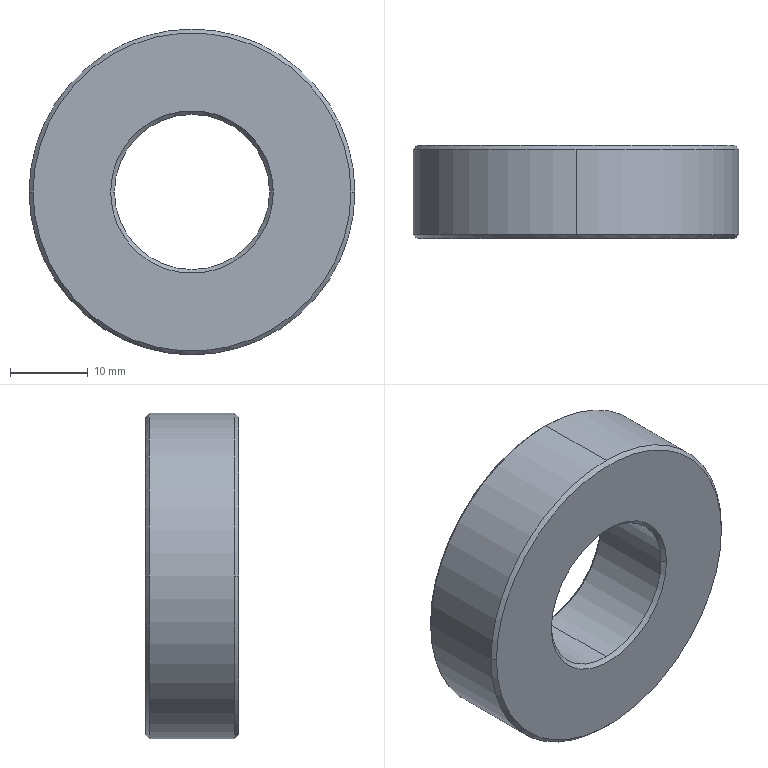Part | SolidWorks | features BaseBody 1 | 1 solid | 14 faces | box 42 x 12 x 42 mm | volume 12807 mm3 | cone 8 | cylinder 4 | plane 2 | commonest cylinder face diameters 20 x2 42 x2
STEP:
#1=CARTESIAN_POINT('',(10.,5.5,0.));
#2=VERTEX_POINT('',#1);
#3=CARTESIAN_POINT('',(0.,5.5,-10.));
#4=VERTEX_POINT('',#3);
#5=CARTESIAN_POINT('',(0.,5.5,0.));
#6=DIRECTION('',(0.,1.,0.));
#7=DIRECTION('',(0.,0.,-1.));
#8=AXIS2_PLACEMENT_3D('',#5,#6,#7);
#9=CIRCLE('',#8,10.);
#10=EDGE_CURVE('',#2,#4,#9,.T.);
#11=ORIENTED_EDGE('',*,*,#10,.F.);
#12=CARTESIAN_POINT('',(10.5,6.,0.));
#13=VERTEX_POINT('',#12);
#14=CARTESIAN_POINT('',(10.5,6.,0.));
#15=DIRECTION('',(0.7071,0.7071,0.));
#16=VECTOR('',#15,1000.);
#17=LINE('',#14,#16);
#18=EDGE_CURVE('',#2,#13,#17,.T.);
#19=ORIENTED_EDGE('',*,*,#18,.T.);
#20=CARTESIAN_POINT('',(-10.5,6.,0.));
#21=VERTEX_POINT('',#20);
#22=CARTESIAN_POINT('',(0.,6.,0.));
#23=DIRECTION('',(0.,-1.,0.));
#24=DIRECTION('',(-1.,0.,0.));
#25=AXIS2_PLACEMENT_3D('',#22,#23,#24);
#26=CIRCLE('',#25,10.5);
#27=EDGE_CURVE('',#21,#13,#26,.T.);
#28=ORIENTED_EDGE('',*,*,#27,.F.);
#29=CARTESIAN_POINT('',(-10.,5.5,0.));
#30=VERTEX_POINT('',#29);
#31=CARTESIAN_POINT('',(-10.5,6.,0.));
#32=DIRECTION('',(-0.7071,0.7071,0.));
#33=VECTOR('',#32,1000.);
#34=LINE('',#31,#33);
#35=EDGE_CURVE('',#30,#21,#34,.T.);
#36=ORIENTED_EDGE('',*,*,#35,.F.);
#37=CARTESIAN_POINT('',(0.,5.5,0.));
#38=DIRECTION('',(0.,1.,0.));
#39=DIRECTION('',(0.,0.,-1.));
#40=AXIS2_PLACEMENT_3D('',#37,#38,#39);
#41=CIRCLE('',#40,10.);
#42=EDGE_CURVE('',#4,#30,#41,.T.);
#43=ORIENTED_EDGE('',*,*,#42,.F.);
#44=EDGE_LOOP('',(#11,#19,#28,#36,#43));
#45=FACE_OUTER_BOUND('',#44,.T.);
#46=CARTESIAN_POINT('',(0.,6.,0.));
#47=DIRECTION('',(0.,1.,0.));
#48=DIRECTION('',(-1.,0.,0.));
#49=AXIS2_PLACEMENT_3D('',#46,#47,#48);
#50=CONICAL_SURFACE('',#49,10.5,0.7854);
#51=ADVANCED_FACE('',(#45),#50,.F.);
#52=CARTESIAN_POINT('',(-20.5,6.,0.));
#53=VERTEX_POINT('',#52);
#54=CARTESIAN_POINT('',(20.5,6.,0.));
#55=VERTEX_POINT('',#54);
#56=CARTESIAN_POINT('',(0.,6.,0.));
#57=DIRECTION('',(0.,1.,0.));
#58=DIRECTION('',(1.,0.,0.));
#59=AXIS2_PLACEMENT_3D('',#56,#57,#58);
#60=CIRCLE('',#59,20.5);
#61=EDGE_CURVE('',#53,#55,#60,.T.);
#62=ORIENTED_EDGE('',*,*,#61,.F.);
#63=CARTESIAN_POINT('',(-21.,5.5,0.));
#64=VERTEX_POINT('',#63);
#65=CARTESIAN_POINT('',(-21.,5.5,0.));
#66=DIRECTION('',(-0.7071,-0.7071,0.));
#67=VECTOR('',#66,1000.);
#68=LINE('',#65,#67);
#69=EDGE_CURVE('',#53,#64,#68,.T.);
#70=ORIENTED_EDGE('',*,*,#69,.T.);
#71=CARTESIAN_POINT('',(0.,5.5,21.));
#72=VERTEX_POINT('',#71);
#73=CARTESIAN_POINT('',(0.,5.5,0.));
#74=DIRECTION('',(0.,1.,0.));
#75=DIRECTION('',(0.,0.,-1.));
#76=AXIS2_PLACEMENT_3D('',#73,#74,#75);
#77=CIRCLE('',#76,21.);
#78=EDGE_CURVE('',#64,#72,#77,.T.);
#79=ORIENTED_EDGE('',*,*,#78,.T.);
#80=CARTESIAN_POINT('',(21.,5.5,0.));
#81=VERTEX_POINT('',#80);
#82=CARTESIAN_POINT('',(0.,5.5,0.));
#83=DIRECTION('',(0.,1.,0.));
#84=DIRECTION('',(0.,0.,-1.));
#85=AXIS2_PLACEMENT_3D('',#82,#83,#84);
#86=CIRCLE('',#85,21.);
#87=EDGE_CURVE('',#72,#81,#86,.T.);
#88=ORIENTED_EDGE('',*,*,#87,.T.);
#89=CARTESIAN_POINT('',(21.,5.5,0.));
#90=DIRECTION('',(0.7071,-0.7071,0.));
#91=VECTOR('',#90,1000.);
#92=LINE('',#89,#91);
#93=EDGE_CURVE('',#55,#81,#92,.T.);
#94=ORIENTED_EDGE('',*,*,#93,.F.);
#95=EDGE_LOOP('',(#62,#70,#79,#88,#94));
#96=FACE_OUTER_BOUND('',#95,.T.);
#97=CARTESIAN_POINT('',(0.,5.5,0.));
#98=DIRECTION('',(0.,-1.,0.));
#99=DIRECTION('',(1.,0.,0.));
#100=AXIS2_PLACEMENT_3D('',#97,#98,#99);
#101=CONICAL_SURFACE('',#100,21.,0.7854);
#102=ADVANCED_FACE('',(#96),#101,.T.);
#103=CARTESIAN_POINT('',(0.,-5.5,-10.));
#104=VERTEX_POINT('',#103);
#105=CARTESIAN_POINT('',(-10.,-5.5,0.));
#106=VERTEX_POINT('',#105);
#107=CARTESIAN_POINT('',(0.,-5.5,0.));
#108=DIRECTION('',(0.,1.,0.));
#109=DIRECTION('',(0.,0.,1.));
#110=AXIS2_PLACEMENT_3D('',#107,#108,#109);
#111=CIRCLE('',#110,10.);
#112=EDGE_CURVE('',#104,#106,#111,.T.);
#113=ORIENTED_EDGE('',*,*,#112,.F.);
#114=CARTESIAN_POINT('',(0.,-6.,-10.));
#115=DIRECTION('',(0.,1.,0.));
#116=VECTOR('',#115,1000.);
#117=LINE('',#114,#116);
#118=EDGE_CURVE('',#104,#4,#117,.T.);
#119=ORIENTED_EDGE('',*,*,#118,.T.);
#120=ORIENTED_EDGE('',*,*,#42,.T.);
#121=CARTESIAN_POINT('',(0.,5.5,10.));
#122=VERTEX_POINT('',#121);
#123=CARTESIAN_POINT('',(0.,5.5,0.));
#124=DIRECTION('',(0.,1.,0.));
#125=DIRECTION('',(0.,0.,-1.));
#126=AXIS2_PLACEMENT_3D('',#123,#124,#125);
#127=CIRCLE('',#126,10.);
#128=EDGE_CURVE('',#30,#122,#127,.T.);
#129=ORIENTED_EDGE('',*,*,#128,.T.);
#130=CARTESIAN_POINT('',(0.,-5.5,10.));
#131=VERTEX_POINT('',#130);
#132=CARTESIAN_POINT('',(0.,-6.,10.));
#133=DIRECTION('',(0.,1.,0.));
#134=VECTOR('',#133,1000.);
#135=LINE('',#132,#134);
#136=EDGE_CURVE('',#131,#122,#135,.T.);
#137=ORIENTED_EDGE('',*,*,#136,.F.);
#138=CARTESIAN_POINT('',(0.,-5.5,0.));
#139=DIRECTION('',(0.,1.,0.));
#140=DIRECTION('',(0.,0.,1.));
#141=AXIS2_PLACEMENT_3D('',#138,#139,#140);
#142=CIRCLE('',#141,10.);
#143=EDGE_CURVE('',#106,#131,#142,.T.);
#144=ORIENTED_EDGE('',*,*,#143,.F.);
#145=EDGE_LOOP('',(#113,#119,#120,#129,#137,#144));
#146=FACE_OUTER_BOUND('',#145,.T.);
#147=CARTESIAN_POINT('',(0.,-6.,0.));
#148=DIRECTION('',(0.,1.,0.));
#149=DIRECTION('',(0.,0.,1.));
#150=AXIS2_PLACEMENT_3D('',#147,#148,#149);
#151=CYLINDRICAL_SURFACE('',#150,10.);
#152=ADVANCED_FACE('',(#146),#151,.F.);
#153=CARTESIAN_POINT('',(21.,-5.5,0.));
#154=VERTEX_POINT('',#153);
#155=CARTESIAN_POINT('',(0.,-5.5,-21.));
#156=VERTEX_POINT('',#155);
#157=CARTESIAN_POINT('',(0.,-5.5,0.));
#158=DIRECTION('',(0.,1.,0.));
#159=DIRECTION('',(0.,0.,1.));
#160=AXIS2_PLACEMENT_3D('',#157,#158,#159);
#161=CIRCLE('',#160,21.);
#162=EDGE_CURVE('',#154,#156,#161,.T.);
#163=ORIENTED_EDGE('',*,*,#162,.T.);
#164=CARTESIAN_POINT('',(0.,5.5,-21.));
#165=VERTEX_POINT('',#164);
#166=CARTESIAN_POINT('',(0.,-6.,-21.));
#167=DIRECTION('',(0.,1.,0.));
#168=VECTOR('',#167,1000.);
#169=LINE('',#166,#168);
#170=EDGE_CURVE('',#156,#165,#169,.T.);
#171=ORIENTED_EDGE('',*,*,#170,.T.);
#172=CARTESIAN_POINT('',(0.,5.5,0.));
#173=DIRECTION('',(0.,1.,0.));
#174=DIRECTION('',(0.,0.,-1.));
#175=AXIS2_PLACEMENT_3D('',#172,#173,#174);
#176=CIRCLE('',#175,21.);
#177=EDGE_CURVE('',#81,#165,#176,.T.);
#178=ORIENTED_EDGE('',*,*,#177,.F.);
#179=ORIENTED_EDGE('',*,*,#87,.F.);
#180=CARTESIAN_POINT('',(0.,-5.5,21.));
#181=VERTEX_POINT('',#180);
#182=CARTESIAN_POINT('',(0.,-6.,21.));
#183=DIRECTION('',(0.,1.,0.));
#184=VECTOR('',#183,1000.);
#185=LINE('',#182,#184);
#186=EDGE_CURVE('',#181,#72,#185,.T.);
#187=ORIENTED_EDGE('',*,*,#186,.F.);
#188=CARTESIAN_POINT('',(0.,-5.5,0.));
#189=DIRECTION('',(0.,1.,0.));
#190=DIRECTION('',(0.,0.,1.));
#191=AXIS2_PLACEMENT_3D('',#188,#189,#190);
#192=CIRCLE('',#191,21.);
#193=EDGE_CURVE('',#181,#154,#192,.T.);
#194=ORIENTED_EDGE('',*,*,#193,.T.);
#195=EDGE_LOOP('',(#163,#171,#178,#179,#187,#194));
#196=FACE_OUTER_BOUND('',#195,.T.);
#197=CARTESIAN_POINT('',(0.,-6.,0.));
#198=DIRECTION('',(0.,1.,0.));
#199=DIRECTION('',(0.,0.,1.));
#200=AXIS2_PLACEMENT_3D('',#197,#198,#199);
#201=CYLINDRICAL_SURFACE('',#200,21.);
#202=ADVANCED_FACE('',(#196),#201,.T.);
#203=CARTESIAN_POINT('',(10.,-5.5,0.));
#204=VERTEX_POINT('',#203);
#205=CARTESIAN_POINT('',(0.,-5.5,0.));
#206=DIRECTION('',(0.,1.,0.));
#207=DIRECTION('',(0.,0.,1.));
#208=AXIS2_PLACEMENT_3D('',#205,#206,#207);
#209=CIRCLE('',#208,10.);
#210=EDGE_CURVE('',#204,#104,#209,.T.);
#211=ORIENTED_EDGE('',*,*,#210,.T.);
#212=ORIENTED_EDGE('',*,*,#112,.T.);
#213=CARTESIAN_POINT('',(-10.5,-6.,0.));
#214=VERTEX_POINT('',#213);
#215=CARTESIAN_POINT('',(-10.5,-6.,0.));
#216=DIRECTION('',(-0.7071,-0.7071,0.));
#217=VECTOR('',#216,1000.);
#218=LINE('',#215,#217);
#219=EDGE_CURVE('',#106,#214,#218,.T.);
#220=ORIENTED_EDGE('',*,*,#219,.T.);
#221=CARTESIAN_POINT('',(10.5,-6.,0.));
#222=VERTEX_POINT('',#221);
#223=CARTESIAN_POINT('',(0.,-6.,0.));
#224=DIRECTION('',(0.,1.,0.));
#225=DIRECTION('',(1.,0.,0.));
#226=AXIS2_PLACEMENT_3D('',#223,#224,#225);
#227=CIRCLE('',#226,10.5);
#228=EDGE_CURVE('',#222,#214,#227,.T.);
#229=ORIENTED_EDGE('',*,*,#228,.F.);
#230=CARTESIAN_POINT('',(10.5,-6.,0.));
#231=DIRECTION('',(0.7071,-0.7071,0.));
#232=VECTOR('',#231,1000.);
#233=LINE('',#230,#232);
#234=EDGE_CURVE('',#204,#222,#233,.T.);
#235=ORIENTED_EDGE('',*,*,#234,.F.);
#236=EDGE_LOOP('',(#211,#212,#220,#229,#235));
#237=FACE_OUTER_BOUND('',#236,.T.);
#238=CARTESIAN_POINT('',(0.,-6.,0.));
#239=DIRECTION('',(0.,-1.,0.));
#240=DIRECTION('',(1.,0.,0.));
#241=AXIS2_PLACEMENT_3D('',#238,#239,#240);
#242=CONICAL_SURFACE('',#241,10.5,0.7854);
#243=ADVANCED_FACE('',(#237),#242,.F.);
#244=CARTESIAN_POINT('',(-20.5,-6.,0.));
#245=VERTEX_POINT('',#244);
#246=CARTESIAN_POINT('',(20.5,-6.,0.));
#247=VERTEX_POINT('',#246);
#248=CARTESIAN_POINT('',(0.,-6.,0.));
#249=DIRECTION('',(0.,1.,0.));
#250=DIRECTION('',(-1.,0.,0.));
#251=AXIS2_PLACEMENT_3D('',#248,#249,#250);
#252=CIRCLE('',#251,20.5);
#253=EDGE_CURVE('',#245,#247,#252,.T.);
#254=ORIENTED_EDGE('',*,*,#253,.T.);
#255=CARTESIAN_POINT('',(21.,-5.5,0.));
#256=DIRECTION('',(0.7071,0.7071,0.));
#257=VECTOR('',#256,1000.);
#258=LINE('',#255,#257);
#259=EDGE_CURVE('',#247,#154,#258,.T.);
#260=ORIENTED_EDGE('',*,*,#259,.T.);
#261=ORIENTED_EDGE('',*,*,#193,.F.);
#262=CARTESIAN_POINT('',(-21.,-5.5,0.));
#263=VERTEX_POINT('',#262);
#264=CARTESIAN_POINT('',(0.,-5.5,0.));
#265=DIRECTION('',(0.,1.,0.));
#266=DIRECTION('',(0.,0.,1.));
#267=AXIS2_PLACEMENT_3D('',#264,#265,#266);
#268=CIRCLE('',#267,21.);
#269=EDGE_CURVE('',#263,#181,#268,.T.);
#270=ORIENTED_EDGE('',*,*,#269,.F.);
#271=CARTESIAN_POINT('',(-21.,-5.5,0.));
#272=DIRECTION('',(-0.7071,0.7071,0.));
#273=VECTOR('',#272,1000.);
#274=LINE('',#271,#273);
#275=EDGE_CURVE('',#245,#263,#274,.T.);
#276=ORIENTED_EDGE('',*,*,#275,.F.);
#277=EDGE_LOOP('',(#254,#260,#261,#270,#276));
#278=FACE_OUTER_BOUND('',#277,.T.);
#279=CARTESIAN_POINT('',(0.,-5.5,0.));
#280=DIRECTION('',(0.,1.,0.));
#281=DIRECTION('',(-1.,0.,0.));
#282=AXIS2_PLACEMENT_3D('',#279,#280,#281);
#283=CONICAL_SURFACE('',#282,21.,0.7854);
#284=ADVANCED_FACE('',(#278),#283,.T.);
#285=ORIENTED_EDGE('',*,*,#27,.T.);
#286=CARTESIAN_POINT('',(0.,6.,0.));
#287=DIRECTION('',(0.,-1.,0.));
#288=DIRECTION('',(-1.,0.,0.));
#289=AXIS2_PLACEMENT_3D('',#286,#287,#288);
#290=CIRCLE('',#289,10.5);
#291=EDGE_CURVE('',#13,#21,#290,.T.);
#292=ORIENTED_EDGE('',*,*,#291,.T.);
#293=EDGE_LOOP('',(#285,#292));
#294=FACE_BOUND('',#293,.T.);
#295=CARTESIAN_POINT('',(0.,6.,0.));
#296=DIRECTION('',(0.,1.,0.));
#297=DIRECTION('',(1.,0.,0.));
#298=AXIS2_PLACEMENT_3D('',#295,#296,#297);
#299=CIRCLE('',#298,20.5);
#300=EDGE_CURVE('',#55,#53,#299,.T.);
#301=ORIENTED_EDGE('',*,*,#300,.T.);
#302=ORIENTED_EDGE('',*,*,#61,.T.);
#303=EDGE_LOOP('',(#301,#302));
#304=FACE_OUTER_BOUND('',#303,.T.);
#305=CARTESIAN_POINT('',(0.,6.,0.));
#306=DIRECTION('',(0.,1.,0.));
#307=DIRECTION('',(0.,0.,1.));
#308=AXIS2_PLACEMENT_3D('',#305,#306,#307);
#309=PLANE('',#308);
#310=ADVANCED_FACE('',(#294,#304),#309,.T.);
#311=ORIENTED_EDGE('',*,*,#18,.F.);
#312=CARTESIAN_POINT('',(0.,5.5,0.));
#313=DIRECTION('',(0.,1.,0.));
#314=DIRECTION('',(0.,0.,-1.));
#315=AXIS2_PLACEMENT_3D('',#312,#313,#314);
#316=CIRCLE('',#315,10.);
#317=EDGE_CURVE('',#122,#2,#316,.T.);
#318=ORIENTED_EDGE('',*,*,#317,.F.);
#319=ORIENTED_EDGE('',*,*,#128,.F.);
#320=ORIENTED_EDGE('',*,*,#35,.T.);
#321=ORIENTED_EDGE('',*,*,#291,.F.);
#322=EDGE_LOOP('',(#311,#318,#319,#320,#321));
#323=FACE_OUTER_BOUND('',#322,.T.);
#324=CARTESIAN_POINT('',(0.,6.,0.));
#325=DIRECTION('',(0.,1.,0.));
#326=DIRECTION('',(-1.,0.,0.));
#327=AXIS2_PLACEMENT_3D('',#324,#325,#326);
#328=CONICAL_SURFACE('',#327,10.5,0.7854);
#329=ADVANCED_FACE('',(#323),#328,.F.);
#330=ORIENTED_EDGE('',*,*,#69,.F.);
#331=ORIENTED_EDGE('',*,*,#300,.F.);
#332=ORIENTED_EDGE('',*,*,#93,.T.);
#333=ORIENTED_EDGE('',*,*,#177,.T.);
#334=CARTESIAN_POINT('',(0.,5.5,0.));
#335=DIRECTION('',(0.,1.,0.));
#336=DIRECTION('',(0.,0.,-1.));
#337=AXIS2_PLACEMENT_3D('',#334,#335,#336);
#338=CIRCLE('',#337,21.);
#339=EDGE_CURVE('',#165,#64,#338,.T.);
#340=ORIENTED_EDGE('',*,*,#339,.T.);
#341=EDGE_LOOP('',(#330,#331,#332,#333,#340));
#342=FACE_OUTER_BOUND('',#341,.T.);
#343=CARTESIAN_POINT('',(0.,5.5,0.));
#344=DIRECTION('',(0.,-1.,0.));
#345=DIRECTION('',(1.,0.,0.));
#346=AXIS2_PLACEMENT_3D('',#343,#344,#345);
#347=CONICAL_SURFACE('',#346,21.,0.7854);
#348=ADVANCED_FACE('',(#342),#347,.T.);
#349=ORIENTED_EDGE('',*,*,#118,.F.);
#350=ORIENTED_EDGE('',*,*,#210,.F.);
#351=CARTESIAN_POINT('',(0.,-5.5,0.));
#352=DIRECTION('',(0.,1.,0.));
#353=DIRECTION('',(0.,0.,1.));
#354=AXIS2_PLACEMENT_3D('',#351,#352,#353);
#355=CIRCLE('',#354,10.);
#356=EDGE_CURVE('',#131,#204,#355,.T.);
#357=ORIENTED_EDGE('',*,*,#356,.F.);
#358=ORIENTED_EDGE('',*,*,#136,.T.);
#359=ORIENTED_EDGE('',*,*,#317,.T.);
#360=ORIENTED_EDGE('',*,*,#10,.T.);
#361=EDGE_LOOP('',(#349,#350,#357,#358,#359,#360));
#362=FACE_OUTER_BOUND('',#361,.T.);
#363=CARTESIAN_POINT('',(0.,-6.,0.));
#364=DIRECTION('',(0.,1.,0.));
#365=DIRECTION('',(0.,0.,1.));
#366=AXIS2_PLACEMENT_3D('',#363,#364,#365);
#367=CYLINDRICAL_SURFACE('',#366,10.);
#368=ADVANCED_FACE('',(#362),#367,.F.);
#369=ORIENTED_EDGE('',*,*,#170,.F.);
#370=CARTESIAN_POINT('',(0.,-5.5,0.));
#371=DIRECTION('',(0.,1.,0.));
#372=DIRECTION('',(0.,0.,1.));
#373=AXIS2_PLACEMENT_3D('',#370,#371,#372);
#374=CIRCLE('',#373,21.);
#375=EDGE_CURVE('',#156,#263,#374,.T.);
#376=ORIENTED_EDGE('',*,*,#375,.T.);
#377=ORIENTED_EDGE('',*,*,#269,.T.);
#378=ORIENTED_EDGE('',*,*,#186,.T.);
#379=ORIENTED_EDGE('',*,*,#78,.F.);
#380=ORIENTED_EDGE('',*,*,#339,.F.);
#381=EDGE_LOOP('',(#369,#376,#377,#378,#379,#380));
#382=FACE_OUTER_BOUND('',#381,.T.);
#383=CARTESIAN_POINT('',(0.,-6.,0.));
#384=DIRECTION('',(0.,1.,0.));
#385=DIRECTION('',(0.,0.,1.));
#386=AXIS2_PLACEMENT_3D('',#383,#384,#385);
#387=CYLINDRICAL_SURFACE('',#386,21.);
#388=ADVANCED_FACE('',(#382),#387,.T.);
#389=ORIENTED_EDGE('',*,*,#219,.F.);
#390=ORIENTED_EDGE('',*,*,#143,.T.);
#391=ORIENTED_EDGE('',*,*,#356,.T.);
#392=ORIENTED_EDGE('',*,*,#234,.T.);
#393=CARTESIAN_POINT('',(0.,-6.,0.));
#394=DIRECTION('',(0.,1.,0.));
#395=DIRECTION('',(1.,0.,0.));
#396=AXIS2_PLACEMENT_3D('',#393,#394,#395);
#397=CIRCLE('',#396,10.5);
#398=EDGE_CURVE('',#214,#222,#397,.T.);
#399=ORIENTED_EDGE('',*,*,#398,.F.);
#400=EDGE_LOOP('',(#389,#390,#391,#392,#399));
#401=FACE_OUTER_BOUND('',#400,.T.);
#402=CARTESIAN_POINT('',(0.,-6.,0.));
#403=DIRECTION('',(0.,-1.,0.));
#404=DIRECTION('',(1.,0.,0.));
#405=AXIS2_PLACEMENT_3D('',#402,#403,#404);
#406=CONICAL_SURFACE('',#405,10.5,0.7854);
#407=ADVANCED_FACE('',(#401),#406,.F.);
#408=ORIENTED_EDGE('',*,*,#259,.F.);
#409=CARTESIAN_POINT('',(0.,-6.,0.));
#410=DIRECTION('',(0.,1.,0.));
#411=DIRECTION('',(-1.,0.,0.));
#412=AXIS2_PLACEMENT_3D('',#409,#410,#411);
#413=CIRCLE('',#412,20.5);
#414=EDGE_CURVE('',#247,#245,#413,.T.);
#415=ORIENTED_EDGE('',*,*,#414,.T.);
#416=ORIENTED_EDGE('',*,*,#275,.T.);
#417=ORIENTED_EDGE('',*,*,#375,.F.);
#418=ORIENTED_EDGE('',*,*,#162,.F.);
#419=EDGE_LOOP('',(#408,#415,#416,#417,#418));
#420=FACE_OUTER_BOUND('',#419,.T.);
#421=CARTESIAN_POINT('',(0.,-5.5,0.));
#422=DIRECTION('',(0.,1.,0.));
#423=DIRECTION('',(-1.,0.,0.));
#424=AXIS2_PLACEMENT_3D('',#421,#422,#423);
#425=CONICAL_SURFACE('',#424,21.,0.7854);
#426=ADVANCED_FACE('',(#420),#425,.T.);
#427=ORIENTED_EDGE('',*,*,#228,.T.);
#428=ORIENTED_EDGE('',*,*,#398,.T.);
#429=EDGE_LOOP('',(#427,#428));
#430=FACE_BOUND('',#429,.T.);
#431=ORIENTED_EDGE('',*,*,#253,.F.);
#432=ORIENTED_EDGE('',*,*,#414,.F.);
#433=EDGE_LOOP('',(#431,#432));
#434=FACE_OUTER_BOUND('',#433,.T.);
#435=CARTESIAN_POINT('',(0.,-6.,0.));
#436=DIRECTION('',(0.,1.,0.));
#437=DIRECTION('',(0.,0.,1.));
#438=AXIS2_PLACEMENT_3D('',#435,#436,#437);
#439=PLANE('',#438);
#440=ADVANCED_FACE('',(#430,#434),#439,.F.);
#441=CLOSED_SHELL('',(#51,#102,#152,#202,#243,#284,#310,#329,#348,#368,#388,#407,#426,#440));
#442=MANIFOLD_SOLID_BREP('',#441);
#443=CARTESIAN_POINT('',(0.,0.,0.));
#444=DIRECTION('',(0.,0.,1.));
#445=DIRECTION('',(1.,0.,0.));
#446=AXIS2_PLACEMENT_3D('',#443,#444,#445);
#447=(LENGTH_UNIT()NAMED_UNIT(*)SI_UNIT(.MILLI.,.METRE.));
#448=UNCERTAINTY_MEASURE_WITH_UNIT(LENGTH_MEASURE(0.00001),#447,'','');
#449=(NAMED_UNIT(*)PLANE_ANGLE_UNIT()SI_UNIT($,.RADIAN.));
#450=(NAMED_UNIT(*)SI_UNIT($,.STERADIAN.)SOLID_ANGLE_UNIT());
#451=(GEOMETRIC_REPRESENTATION_CONTEXT(3)GLOBAL_UNCERTAINTY_ASSIGNED_CONTEXT((#448))GLOBAL_UNIT_ASSIGNED_CONTEXT((#447,#449,#450))REPRESENTATION_CONTEXT('',''));
#452=ADVANCED_BREP_SHAPE_REPRESENTATION('',(#442,#446),#451);